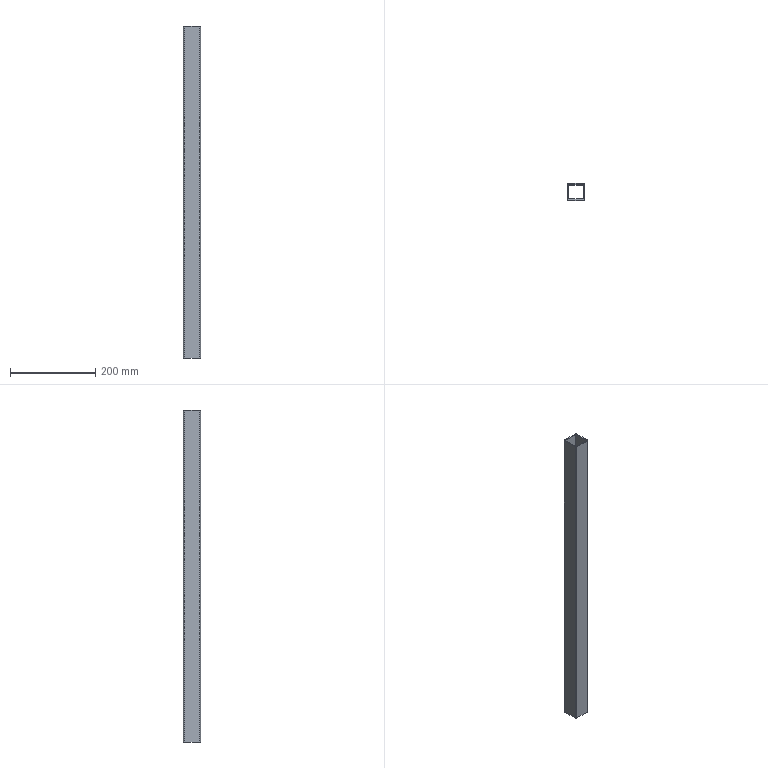Part | STEP file | X77-03116 | 1 solid | 14 faces | box 40 x 40 x 780 mm | volume 340294 mm3 | plane 10 | cylinder 4 | commonest cylinder face diameters 6 x4
STEP:
#1=CARTESIAN_POINT('',(-20.,-17.,780.));
#2=VERTEX_POINT('',#1);
#3=CARTESIAN_POINT('',(-17.,-20.,780.));
#4=VERTEX_POINT('',#3);
#5=CARTESIAN_POINT('',(-17.,-17.,780.));
#6=DIRECTION('',(0.,0.,1.));
#7=DIRECTION('',(-1.,0.,0.));
#8=AXIS2_PLACEMENT_3D('',#5,#6,#7);
#9=CIRCLE('',#8,3.);
#10=EDGE_CURVE('',#2,#4,#9,.T.);
#11=ORIENTED_EDGE('',*,*,#10,.T.);
#12=CARTESIAN_POINT('',(17.,-20.,780.));
#13=VERTEX_POINT('',#12);
#14=CARTESIAN_POINT('',(-17.,-20.,780.));
#15=DIRECTION('',(1.,0.,0.));
#16=VECTOR('',#15,1000.);
#17=LINE('',#14,#16);
#18=EDGE_CURVE('',#4,#13,#17,.T.);
#19=ORIENTED_EDGE('',*,*,#18,.T.);
#20=CARTESIAN_POINT('',(20.,-17.,780.));
#21=VERTEX_POINT('',#20);
#22=CARTESIAN_POINT('',(17.,-17.,780.));
#23=DIRECTION('',(0.,0.,1.));
#24=DIRECTION('',(-1.,0.,0.));
#25=AXIS2_PLACEMENT_3D('',#22,#23,#24);
#26=CIRCLE('',#25,3.);
#27=EDGE_CURVE('',#13,#21,#26,.T.);
#28=ORIENTED_EDGE('',*,*,#27,.T.);
#29=CARTESIAN_POINT('',(20.,17.,780.));
#30=VERTEX_POINT('',#29);
#31=CARTESIAN_POINT('',(20.,-17.,780.));
#32=DIRECTION('',(0.,1.,0.));
#33=VECTOR('',#32,1000.);
#34=LINE('',#31,#33);
#35=EDGE_CURVE('',#21,#30,#34,.T.);
#36=ORIENTED_EDGE('',*,*,#35,.T.);
#37=CARTESIAN_POINT('',(17.,20.,780.));
#38=VERTEX_POINT('',#37);
#39=CARTESIAN_POINT('',(17.,17.,780.));
#40=DIRECTION('',(0.,0.,1.));
#41=DIRECTION('',(1.,0.,0.));
#42=AXIS2_PLACEMENT_3D('',#39,#40,#41);
#43=CIRCLE('',#42,3.);
#44=EDGE_CURVE('',#30,#38,#43,.T.);
#45=ORIENTED_EDGE('',*,*,#44,.T.);
#46=CARTESIAN_POINT('',(-17.,20.,780.));
#47=VERTEX_POINT('',#46);
#48=CARTESIAN_POINT('',(-17.,20.,780.));
#49=DIRECTION('',(-1.,0.,0.));
#50=VECTOR('',#49,1000.);
#51=LINE('',#48,#50);
#52=EDGE_CURVE('',#38,#47,#51,.T.);
#53=ORIENTED_EDGE('',*,*,#52,.T.);
#54=CARTESIAN_POINT('',(-20.,17.,780.));
#55=VERTEX_POINT('',#54);
#56=CARTESIAN_POINT('',(-17.,17.,780.));
#57=DIRECTION('',(0.,0.,1.));
#58=DIRECTION('',(1.,0.,0.));
#59=AXIS2_PLACEMENT_3D('',#56,#57,#58);
#60=CIRCLE('',#59,3.);
#61=EDGE_CURVE('',#47,#55,#60,.T.);
#62=ORIENTED_EDGE('',*,*,#61,.T.);
#63=CARTESIAN_POINT('',(-20.,-17.,780.));
#64=DIRECTION('',(0.,-1.,0.));
#65=VECTOR('',#64,1000.);
#66=LINE('',#63,#65);
#67=EDGE_CURVE('',#55,#2,#66,.T.);
#68=ORIENTED_EDGE('',*,*,#67,.T.);
#69=EDGE_LOOP('',(#11,#19,#28,#36,#45,#53,#62,#68));
#70=FACE_OUTER_BOUND('',#69,.T.);
#71=CARTESIAN_POINT('',(17.,-17.,780.));
#72=VERTEX_POINT('',#71);
#73=CARTESIAN_POINT('',(17.,17.,780.));
#74=VERTEX_POINT('',#73);
#75=CARTESIAN_POINT('',(17.,-17.,780.));
#76=DIRECTION('',(0.,1.,0.));
#77=VECTOR('',#76,1000.);
#78=LINE('',#75,#77);
#79=EDGE_CURVE('',#72,#74,#78,.T.);
#80=ORIENTED_EDGE('',*,*,#79,.F.);
#81=CARTESIAN_POINT('',(-17.,-17.,780.));
#82=VERTEX_POINT('',#81);
#83=CARTESIAN_POINT('',(-17.,-17.,780.));
#84=DIRECTION('',(1.,0.,0.));
#85=VECTOR('',#84,1000.);
#86=LINE('',#83,#85);
#87=EDGE_CURVE('',#82,#72,#86,.T.);
#88=ORIENTED_EDGE('',*,*,#87,.F.);
#89=CARTESIAN_POINT('',(-17.,17.,780.));
#90=VERTEX_POINT('',#89);
#91=CARTESIAN_POINT('',(-17.,-17.,780.));
#92=DIRECTION('',(0.,-1.,0.));
#93=VECTOR('',#92,1000.);
#94=LINE('',#91,#93);
#95=EDGE_CURVE('',#90,#82,#94,.T.);
#96=ORIENTED_EDGE('',*,*,#95,.F.);
#97=CARTESIAN_POINT('',(-17.,17.,780.));
#98=DIRECTION('',(-1.,0.,0.));
#99=VECTOR('',#98,1000.);
#100=LINE('',#97,#99);
#101=EDGE_CURVE('',#74,#90,#100,.T.);
#102=ORIENTED_EDGE('',*,*,#101,.F.);
#103=EDGE_LOOP('',(#80,#88,#96,#102));
#104=FACE_BOUND('',#103,.T.);
#105=CARTESIAN_POINT('',(-17.,-17.,780.));
#106=DIRECTION('',(0.,0.,-1.));
#107=DIRECTION('',(-1.,0.,0.));
#108=AXIS2_PLACEMENT_3D('',#105,#106,#107);
#109=PLANE('',#108);
#110=ADVANCED_FACE('',(#70,#104),#109,.F.);
#111=CARTESIAN_POINT('',(-20.,-17.,0.));
#112=VERTEX_POINT('',#111);
#113=CARTESIAN_POINT('',(-17.,-20.,0.));
#114=VERTEX_POINT('',#113);
#115=CARTESIAN_POINT('',(-17.,-17.,0.));
#116=DIRECTION('',(0.,0.,1.));
#117=DIRECTION('',(-1.,0.,0.));
#118=AXIS2_PLACEMENT_3D('',#115,#116,#117);
#119=CIRCLE('',#118,3.);
#120=EDGE_CURVE('',#112,#114,#119,.T.);
#121=ORIENTED_EDGE('',*,*,#120,.F.);
#122=CARTESIAN_POINT('',(-20.,17.,0.));
#123=VERTEX_POINT('',#122);
#124=CARTESIAN_POINT('',(-20.,-17.,0.));
#125=DIRECTION('',(0.,-1.,0.));
#126=VECTOR('',#125,1000.);
#127=LINE('',#124,#126);
#128=EDGE_CURVE('',#123,#112,#127,.T.);
#129=ORIENTED_EDGE('',*,*,#128,.F.);
#130=CARTESIAN_POINT('',(-17.,20.,0.));
#131=VERTEX_POINT('',#130);
#132=CARTESIAN_POINT('',(-17.,17.,0.));
#133=DIRECTION('',(0.,0.,1.));
#134=DIRECTION('',(1.,0.,0.));
#135=AXIS2_PLACEMENT_3D('',#132,#133,#134);
#136=CIRCLE('',#135,3.);
#137=EDGE_CURVE('',#131,#123,#136,.T.);
#138=ORIENTED_EDGE('',*,*,#137,.F.);
#139=CARTESIAN_POINT('',(17.,20.,0.));
#140=VERTEX_POINT('',#139);
#141=CARTESIAN_POINT('',(-17.,20.,0.));
#142=DIRECTION('',(-1.,0.,0.));
#143=VECTOR('',#142,1000.);
#144=LINE('',#141,#143);
#145=EDGE_CURVE('',#140,#131,#144,.T.);
#146=ORIENTED_EDGE('',*,*,#145,.F.);
#147=CARTESIAN_POINT('',(20.,17.,0.));
#148=VERTEX_POINT('',#147);
#149=CARTESIAN_POINT('',(17.,17.,0.));
#150=DIRECTION('',(0.,0.,1.));
#151=DIRECTION('',(1.,0.,0.));
#152=AXIS2_PLACEMENT_3D('',#149,#150,#151);
#153=CIRCLE('',#152,3.);
#154=EDGE_CURVE('',#148,#140,#153,.T.);
#155=ORIENTED_EDGE('',*,*,#154,.F.);
#156=CARTESIAN_POINT('',(20.,-17.,0.));
#157=VERTEX_POINT('',#156);
#158=CARTESIAN_POINT('',(20.,-17.,0.));
#159=DIRECTION('',(0.,1.,0.));
#160=VECTOR('',#159,1000.);
#161=LINE('',#158,#160);
#162=EDGE_CURVE('',#157,#148,#161,.T.);
#163=ORIENTED_EDGE('',*,*,#162,.F.);
#164=CARTESIAN_POINT('',(17.,-20.,0.));
#165=VERTEX_POINT('',#164);
#166=CARTESIAN_POINT('',(17.,-17.,0.));
#167=DIRECTION('',(0.,0.,1.));
#168=DIRECTION('',(-1.,0.,0.));
#169=AXIS2_PLACEMENT_3D('',#166,#167,#168);
#170=CIRCLE('',#169,3.);
#171=EDGE_CURVE('',#165,#157,#170,.T.);
#172=ORIENTED_EDGE('',*,*,#171,.F.);
#173=CARTESIAN_POINT('',(-17.,-20.,0.));
#174=DIRECTION('',(1.,0.,0.));
#175=VECTOR('',#174,1000.);
#176=LINE('',#173,#175);
#177=EDGE_CURVE('',#114,#165,#176,.T.);
#178=ORIENTED_EDGE('',*,*,#177,.F.);
#179=EDGE_LOOP('',(#121,#129,#138,#146,#155,#163,#172,#178));
#180=FACE_OUTER_BOUND('',#179,.T.);
#181=CARTESIAN_POINT('',(-17.,-17.,0.));
#182=VERTEX_POINT('',#181);
#183=CARTESIAN_POINT('',(17.,-17.,0.));
#184=VERTEX_POINT('',#183);
#185=CARTESIAN_POINT('',(-17.,-17.,0.));
#186=DIRECTION('',(1.,0.,0.));
#187=VECTOR('',#186,1000.);
#188=LINE('',#185,#187);
#189=EDGE_CURVE('',#182,#184,#188,.T.);
#190=ORIENTED_EDGE('',*,*,#189,.T.);
#191=CARTESIAN_POINT('',(17.,17.,0.));
#192=VERTEX_POINT('',#191);
#193=CARTESIAN_POINT('',(17.,-17.,0.));
#194=DIRECTION('',(0.,1.,0.));
#195=VECTOR('',#194,1000.);
#196=LINE('',#193,#195);
#197=EDGE_CURVE('',#184,#192,#196,.T.);
#198=ORIENTED_EDGE('',*,*,#197,.T.);
#199=CARTESIAN_POINT('',(-17.,17.,0.));
#200=VERTEX_POINT('',#199);
#201=CARTESIAN_POINT('',(-17.,17.,0.));
#202=DIRECTION('',(-1.,0.,0.));
#203=VECTOR('',#202,1000.);
#204=LINE('',#201,#203);
#205=EDGE_CURVE('',#192,#200,#204,.T.);
#206=ORIENTED_EDGE('',*,*,#205,.T.);
#207=CARTESIAN_POINT('',(-17.,-17.,0.));
#208=DIRECTION('',(0.,-1.,0.));
#209=VECTOR('',#208,1000.);
#210=LINE('',#207,#209);
#211=EDGE_CURVE('',#200,#182,#210,.T.);
#212=ORIENTED_EDGE('',*,*,#211,.T.);
#213=EDGE_LOOP('',(#190,#198,#206,#212));
#214=FACE_BOUND('',#213,.T.);
#215=CARTESIAN_POINT('',(-17.,-17.,0.));
#216=DIRECTION('',(0.,0.,-1.));
#217=DIRECTION('',(-1.,0.,0.));
#218=AXIS2_PLACEMENT_3D('',#215,#216,#217);
#219=PLANE('',#218);
#220=ADVANCED_FACE('',(#180,#214),#219,.T.);
#221=ORIENTED_EDGE('',*,*,#120,.T.);
#222=CARTESIAN_POINT('',(-17.,-20.,780.));
#223=DIRECTION('',(0.,0.,-1.));
#224=VECTOR('',#223,1000.);
#225=LINE('',#222,#224);
#226=EDGE_CURVE('',#4,#114,#225,.T.);
#227=ORIENTED_EDGE('',*,*,#226,.F.);
#228=ORIENTED_EDGE('',*,*,#10,.F.);
#229=CARTESIAN_POINT('',(-20.,-17.,780.));
#230=DIRECTION('',(0.,0.,-1.));
#231=VECTOR('',#230,1000.);
#232=LINE('',#229,#231);
#233=EDGE_CURVE('',#2,#112,#232,.T.);
#234=ORIENTED_EDGE('',*,*,#233,.T.);
#235=EDGE_LOOP('',(#221,#227,#228,#234));
#236=FACE_OUTER_BOUND('',#235,.T.);
#237=CARTESIAN_POINT('',(-17.,-17.,780.));
#238=DIRECTION('',(0.,0.,-1.));
#239=DIRECTION('',(-1.,0.,0.));
#240=AXIS2_PLACEMENT_3D('',#237,#238,#239);
#241=CYLINDRICAL_SURFACE('',#240,3.);
#242=ADVANCED_FACE('',(#236),#241,.T.);
#243=ORIENTED_EDGE('',*,*,#177,.T.);
#244=CARTESIAN_POINT('',(17.,-20.,780.));
#245=DIRECTION('',(0.,0.,-1.));
#246=VECTOR('',#245,1000.);
#247=LINE('',#244,#246);
#248=EDGE_CURVE('',#13,#165,#247,.T.);
#249=ORIENTED_EDGE('',*,*,#248,.F.);
#250=ORIENTED_EDGE('',*,*,#18,.F.);
#251=ORIENTED_EDGE('',*,*,#226,.T.);
#252=EDGE_LOOP('',(#243,#249,#250,#251));
#253=FACE_OUTER_BOUND('',#252,.T.);
#254=CARTESIAN_POINT('',(-17.,-20.,780.));
#255=DIRECTION('',(0.,1.,0.));
#256=DIRECTION('',(0.,0.,1.));
#257=AXIS2_PLACEMENT_3D('',#254,#255,#256);
#258=PLANE('',#257);
#259=ADVANCED_FACE('',(#253),#258,.F.);
#260=ORIENTED_EDGE('',*,*,#171,.T.);
#261=CARTESIAN_POINT('',(20.,-17.,780.));
#262=DIRECTION('',(0.,0.,-1.));
#263=VECTOR('',#262,1000.);
#264=LINE('',#261,#263);
#265=EDGE_CURVE('',#21,#157,#264,.T.);
#266=ORIENTED_EDGE('',*,*,#265,.F.);
#267=ORIENTED_EDGE('',*,*,#27,.F.);
#268=ORIENTED_EDGE('',*,*,#248,.T.);
#269=EDGE_LOOP('',(#260,#266,#267,#268));
#270=FACE_OUTER_BOUND('',#269,.T.);
#271=CARTESIAN_POINT('',(17.,-17.,780.));
#272=DIRECTION('',(0.,0.,-1.));
#273=DIRECTION('',(-1.,0.,0.));
#274=AXIS2_PLACEMENT_3D('',#271,#272,#273);
#275=CYLINDRICAL_SURFACE('',#274,3.);
#276=ADVANCED_FACE('',(#270),#275,.T.);
#277=ORIENTED_EDGE('',*,*,#162,.T.);
#278=CARTESIAN_POINT('',(20.,17.,780.));
#279=DIRECTION('',(0.,0.,-1.));
#280=VECTOR('',#279,1000.);
#281=LINE('',#278,#280);
#282=EDGE_CURVE('',#30,#148,#281,.T.);
#283=ORIENTED_EDGE('',*,*,#282,.F.);
#284=ORIENTED_EDGE('',*,*,#35,.F.);
#285=ORIENTED_EDGE('',*,*,#265,.T.);
#286=EDGE_LOOP('',(#277,#283,#284,#285));
#287=FACE_OUTER_BOUND('',#286,.T.);
#288=CARTESIAN_POINT('',(20.,-17.,780.));
#289=DIRECTION('',(-1.,0.,0.));
#290=DIRECTION('',(0.,0.,1.));
#291=AXIS2_PLACEMENT_3D('',#288,#289,#290);
#292=PLANE('',#291);
#293=ADVANCED_FACE('',(#287),#292,.F.);
#294=ORIENTED_EDGE('',*,*,#154,.T.);
#295=CARTESIAN_POINT('',(17.,20.,780.));
#296=DIRECTION('',(0.,0.,-1.));
#297=VECTOR('',#296,1000.);
#298=LINE('',#295,#297);
#299=EDGE_CURVE('',#38,#140,#298,.T.);
#300=ORIENTED_EDGE('',*,*,#299,.F.);
#301=ORIENTED_EDGE('',*,*,#44,.F.);
#302=ORIENTED_EDGE('',*,*,#282,.T.);
#303=EDGE_LOOP('',(#294,#300,#301,#302));
#304=FACE_OUTER_BOUND('',#303,.T.);
#305=CARTESIAN_POINT('',(17.,17.,780.));
#306=DIRECTION('',(0.,0.,-1.));
#307=DIRECTION('',(-1.,0.,0.));
#308=AXIS2_PLACEMENT_3D('',#305,#306,#307);
#309=CYLINDRICAL_SURFACE('',#308,3.);
#310=ADVANCED_FACE('',(#304),#309,.T.);
#311=ORIENTED_EDGE('',*,*,#145,.T.);
#312=CARTESIAN_POINT('',(-17.,20.,780.));
#313=DIRECTION('',(0.,0.,-1.));
#314=VECTOR('',#313,1000.);
#315=LINE('',#312,#314);
#316=EDGE_CURVE('',#47,#131,#315,.T.);
#317=ORIENTED_EDGE('',*,*,#316,.F.);
#318=ORIENTED_EDGE('',*,*,#52,.F.);
#319=ORIENTED_EDGE('',*,*,#299,.T.);
#320=EDGE_LOOP('',(#311,#317,#318,#319));
#321=FACE_OUTER_BOUND('',#320,.T.);
#322=CARTESIAN_POINT('',(-17.,20.,780.));
#323=DIRECTION('',(0.,-1.,0.));
#324=DIRECTION('',(0.,0.,-1.));
#325=AXIS2_PLACEMENT_3D('',#322,#323,#324);
#326=PLANE('',#325);
#327=ADVANCED_FACE('',(#321),#326,.F.);
#328=ORIENTED_EDGE('',*,*,#137,.T.);
#329=CARTESIAN_POINT('',(-20.,17.,780.));
#330=DIRECTION('',(0.,0.,-1.));
#331=VECTOR('',#330,1000.);
#332=LINE('',#329,#331);
#333=EDGE_CURVE('',#55,#123,#332,.T.);
#334=ORIENTED_EDGE('',*,*,#333,.F.);
#335=ORIENTED_EDGE('',*,*,#61,.F.);
#336=ORIENTED_EDGE('',*,*,#316,.T.);
#337=EDGE_LOOP('',(#328,#334,#335,#336));
#338=FACE_OUTER_BOUND('',#337,.T.);
#339=CARTESIAN_POINT('',(-17.,17.,780.));
#340=DIRECTION('',(0.,0.,-1.));
#341=DIRECTION('',(-1.,0.,0.));
#342=AXIS2_PLACEMENT_3D('',#339,#340,#341);
#343=CYLINDRICAL_SURFACE('',#342,3.);
#344=ADVANCED_FACE('',(#338),#343,.T.);
#345=ORIENTED_EDGE('',*,*,#128,.T.);
#346=ORIENTED_EDGE('',*,*,#233,.F.);
#347=ORIENTED_EDGE('',*,*,#67,.F.);
#348=ORIENTED_EDGE('',*,*,#333,.T.);
#349=EDGE_LOOP('',(#345,#346,#347,#348));
#350=FACE_OUTER_BOUND('',#349,.T.);
#351=CARTESIAN_POINT('',(-20.,-17.,780.));
#352=DIRECTION('',(1.,0.,0.));
#353=DIRECTION('',(0.,0.,-1.));
#354=AXIS2_PLACEMENT_3D('',#351,#352,#353);
#355=PLANE('',#354);
#356=ADVANCED_FACE('',(#350),#355,.F.);
#357=ORIENTED_EDGE('',*,*,#197,.F.);
#358=CARTESIAN_POINT('',(17.,-17.,780.));
#359=DIRECTION('',(0.,0.,-1.));
#360=VECTOR('',#359,1000.);
#361=LINE('',#358,#360);
#362=EDGE_CURVE('',#72,#184,#361,.T.);
#363=ORIENTED_EDGE('',*,*,#362,.F.);
#364=ORIENTED_EDGE('',*,*,#79,.T.);
#365=CARTESIAN_POINT('',(17.,17.,780.));
#366=DIRECTION('',(0.,0.,-1.));
#367=VECTOR('',#366,1000.);
#368=LINE('',#365,#367);
#369=EDGE_CURVE('',#74,#192,#368,.T.);
#370=ORIENTED_EDGE('',*,*,#369,.T.);
#371=EDGE_LOOP('',(#357,#363,#364,#370));
#372=FACE_OUTER_BOUND('',#371,.T.);
#373=CARTESIAN_POINT('',(17.,-17.,780.));
#374=DIRECTION('',(-1.,0.,0.));
#375=DIRECTION('',(0.,0.,1.));
#376=AXIS2_PLACEMENT_3D('',#373,#374,#375);
#377=PLANE('',#376);
#378=ADVANCED_FACE('',(#372),#377,.T.);
#379=ORIENTED_EDGE('',*,*,#205,.F.);
#380=ORIENTED_EDGE('',*,*,#369,.F.);
#381=ORIENTED_EDGE('',*,*,#101,.T.);
#382=CARTESIAN_POINT('',(-17.,17.,780.));
#383=DIRECTION('',(0.,0.,-1.));
#384=VECTOR('',#383,1000.);
#385=LINE('',#382,#384);
#386=EDGE_CURVE('',#90,#200,#385,.T.);
#387=ORIENTED_EDGE('',*,*,#386,.T.);
#388=EDGE_LOOP('',(#379,#380,#381,#387));
#389=FACE_OUTER_BOUND('',#388,.T.);
#390=CARTESIAN_POINT('',(-17.,17.,780.));
#391=DIRECTION('',(0.,-1.,0.));
#392=DIRECTION('',(0.,0.,-1.));
#393=AXIS2_PLACEMENT_3D('',#390,#391,#392);
#394=PLANE('',#393);
#395=ADVANCED_FACE('',(#389),#394,.T.);
#396=ORIENTED_EDGE('',*,*,#211,.F.);
#397=ORIENTED_EDGE('',*,*,#386,.F.);
#398=ORIENTED_EDGE('',*,*,#95,.T.);
#399=CARTESIAN_POINT('',(-17.,-17.,780.));
#400=DIRECTION('',(0.,0.,-1.));
#401=VECTOR('',#400,1000.);
#402=LINE('',#399,#401);
#403=EDGE_CURVE('',#82,#182,#402,.T.);
#404=ORIENTED_EDGE('',*,*,#403,.T.);
#405=EDGE_LOOP('',(#396,#397,#398,#404));
#406=FACE_OUTER_BOUND('',#405,.T.);
#407=CARTESIAN_POINT('',(-17.,-17.,780.));
#408=DIRECTION('',(1.,0.,0.));
#409=DIRECTION('',(0.,0.,-1.));
#410=AXIS2_PLACEMENT_3D('',#407,#408,#409);
#411=PLANE('',#410);
#412=ADVANCED_FACE('',(#406),#411,.T.);
#413=ORIENTED_EDGE('',*,*,#189,.F.);
#414=ORIENTED_EDGE('',*,*,#403,.F.);
#415=ORIENTED_EDGE('',*,*,#87,.T.);
#416=ORIENTED_EDGE('',*,*,#362,.T.);
#417=EDGE_LOOP('',(#413,#414,#415,#416));
#418=FACE_OUTER_BOUND('',#417,.T.);
#419=CARTESIAN_POINT('',(-17.,-17.,780.));
#420=DIRECTION('',(0.,1.,0.));
#421=DIRECTION('',(0.,0.,1.));
#422=AXIS2_PLACEMENT_3D('',#419,#420,#421);
#423=PLANE('',#422);
#424=ADVANCED_FACE('',(#418),#423,.T.);
#425=CLOSED_SHELL('',(#110,#220,#242,#259,#276,#293,#310,#327,#344,#356,#378,#395,#412,#424));
#426=MANIFOLD_SOLID_BREP('',#425);
#427=CARTESIAN_POINT('',(0.,0.,0.));
#428=DIRECTION('',(0.,0.,1.));
#429=DIRECTION('',(1.,0.,0.));
#430=AXIS2_PLACEMENT_3D('',#427,#428,#429);
#431=(LENGTH_UNIT()NAMED_UNIT(*)SI_UNIT(.MILLI.,.METRE.));
#432=UNCERTAINTY_MEASURE_WITH_UNIT(LENGTH_MEASURE(0.00001),#431,'','');
#433=(NAMED_UNIT(*)PLANE_ANGLE_UNIT()SI_UNIT($,.RADIAN.));
#434=(NAMED_UNIT(*)SI_UNIT($,.STERADIAN.)SOLID_ANGLE_UNIT());
#435=(GEOMETRIC_REPRESENTATION_CONTEXT(3)GLOBAL_UNCERTAINTY_ASSIGNED_CONTEXT((#432))GLOBAL_UNIT_ASSIGNED_CONTEXT((#431,#433,#434))REPRESENTATION_CONTEXT('',''));
#436=ADVANCED_BREP_SHAPE_REPRESENTATION('',(#426,#430),#435);